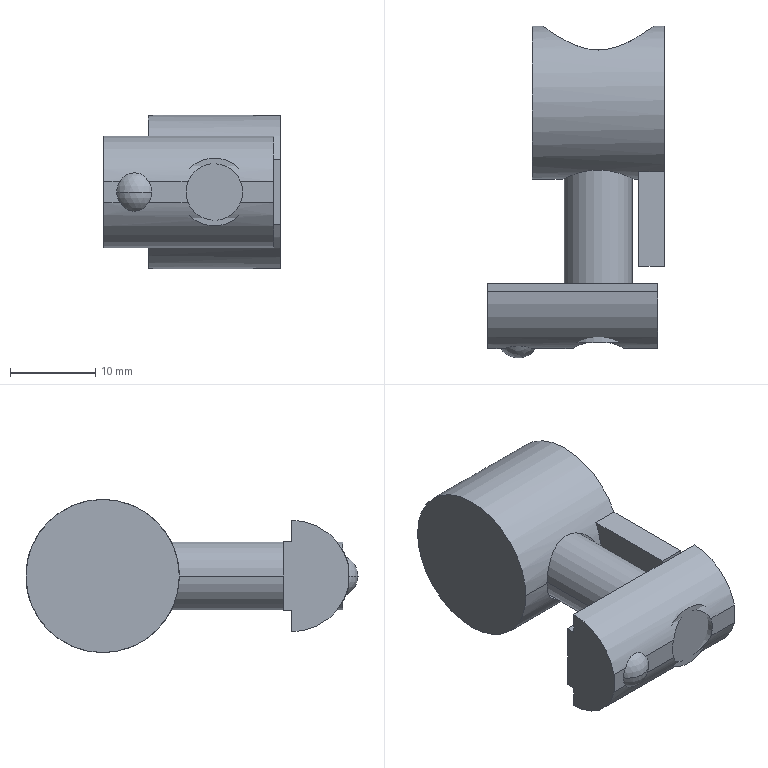Part | STEP file | 3 solids | 52 faces | box 20.75 x 39 x 18 mm | volume 5675 mm3 | plane 32 | cylinder 14 | cone 2 | torus 2 | sphere 2 | commonest cylinder face diameters 13.1 x4 6.647 x2 8 x2 8.5 x2 13.77 x2 18 x2